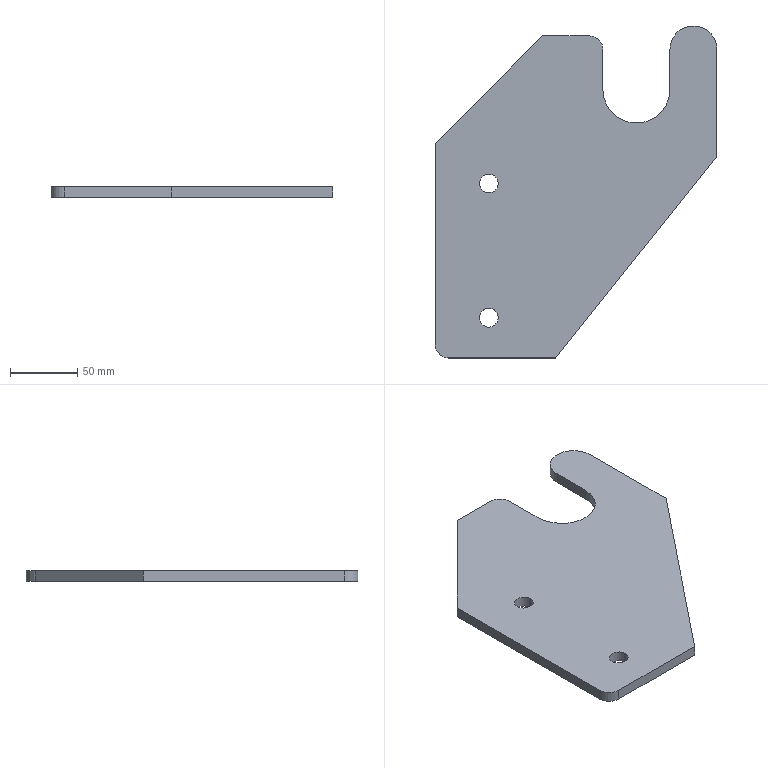Part | SolidWorks | features Extrusion 1 | 1 solid | 18 faces | box 210 x 247.5 x 8 mm | volume 279988 mm3 | plane 10 | cylinder 8 | commonest cylinder face diameters 14 x4 20 x2 35 x1 50 x1
STEP:
#1=CARTESIAN_POINT('',(33.,30.,8.));
#2=VERTEX_POINT('',#1);
#3=CARTESIAN_POINT('',(47.,30.,8.));
#4=VERTEX_POINT('',#3);
#5=CARTESIAN_POINT('',(40.,30.,8.));
#6=DIRECTION('',(0.,0.,1.));
#7=DIRECTION('',(1.,0.,0.));
#8=AXIS2_PLACEMENT_3D('',#5,#6,#7);
#9=CIRCLE('',#8,7.);
#10=EDGE_CURVE('',#2,#4,#9,.T.);
#11=ORIENTED_EDGE('',*,*,#10,.T.);
#12=CARTESIAN_POINT('',(47.,30.,0.));
#13=VERTEX_POINT('',#12);
#14=CARTESIAN_POINT('',(47.,30.,8.));
#15=DIRECTION('',(0.,0.,-1.));
#16=VECTOR('',#15,1000.);
#17=LINE('',#14,#16);
#18=EDGE_CURVE('',#4,#13,#17,.T.);
#19=ORIENTED_EDGE('',*,*,#18,.T.);
#20=CARTESIAN_POINT('',(33.,30.,0.));
#21=VERTEX_POINT('',#20);
#22=CARTESIAN_POINT('',(40.,30.,0.));
#23=DIRECTION('',(0.,0.,1.));
#24=DIRECTION('',(1.,0.,0.));
#25=AXIS2_PLACEMENT_3D('',#22,#23,#24);
#26=CIRCLE('',#25,7.);
#27=EDGE_CURVE('',#21,#13,#26,.T.);
#28=ORIENTED_EDGE('',*,*,#27,.F.);
#29=CARTESIAN_POINT('',(33.,30.,8.));
#30=DIRECTION('',(0.,0.,-1.));
#31=VECTOR('',#30,1000.);
#32=LINE('',#29,#31);
#33=EDGE_CURVE('',#2,#21,#32,.T.);
#34=ORIENTED_EDGE('',*,*,#33,.F.);
#35=EDGE_LOOP('',(#11,#19,#28,#34));
#36=FACE_OUTER_BOUND('',#35,.T.);
#37=CARTESIAN_POINT('',(40.,30.,8.));
#38=DIRECTION('',(0.,0.,-1.));
#39=DIRECTION('',(-1.,0.,0.));
#40=AXIS2_PLACEMENT_3D('',#37,#38,#39);
#41=CYLINDRICAL_SURFACE('',#40,7.);
#42=ADVANCED_FACE('',(#36),#41,.F.);
#43=CARTESIAN_POINT('',(33.,130.,8.));
#44=VERTEX_POINT('',#43);
#45=CARTESIAN_POINT('',(47.,130.,8.));
#46=VERTEX_POINT('',#45);
#47=CARTESIAN_POINT('',(40.,130.,8.));
#48=DIRECTION('',(0.,0.,1.));
#49=DIRECTION('',(1.,0.,0.));
#50=AXIS2_PLACEMENT_3D('',#47,#48,#49);
#51=CIRCLE('',#50,7.);
#52=EDGE_CURVE('',#44,#46,#51,.T.);
#53=ORIENTED_EDGE('',*,*,#52,.T.);
#54=CARTESIAN_POINT('',(47.,130.,0.));
#55=VERTEX_POINT('',#54);
#56=CARTESIAN_POINT('',(47.,130.,8.));
#57=DIRECTION('',(0.,0.,-1.));
#58=VECTOR('',#57,1000.);
#59=LINE('',#56,#58);
#60=EDGE_CURVE('',#46,#55,#59,.T.);
#61=ORIENTED_EDGE('',*,*,#60,.T.);
#62=CARTESIAN_POINT('',(33.,130.,0.));
#63=VERTEX_POINT('',#62);
#64=CARTESIAN_POINT('',(40.,130.,0.));
#65=DIRECTION('',(0.,0.,1.));
#66=DIRECTION('',(1.,0.,0.));
#67=AXIS2_PLACEMENT_3D('',#64,#65,#66);
#68=CIRCLE('',#67,7.);
#69=EDGE_CURVE('',#63,#55,#68,.T.);
#70=ORIENTED_EDGE('',*,*,#69,.F.);
#71=CARTESIAN_POINT('',(33.,130.,8.));
#72=DIRECTION('',(0.,0.,-1.));
#73=VECTOR('',#72,1000.);
#74=LINE('',#71,#73);
#75=EDGE_CURVE('',#44,#63,#74,.T.);
#76=ORIENTED_EDGE('',*,*,#75,.F.);
#77=EDGE_LOOP('',(#53,#61,#70,#76));
#78=FACE_OUTER_BOUND('',#77,.T.);
#79=CARTESIAN_POINT('',(40.,130.,8.));
#80=DIRECTION('',(0.,0.,-1.));
#81=DIRECTION('',(-1.,0.,0.));
#82=AXIS2_PLACEMENT_3D('',#79,#80,#81);
#83=CYLINDRICAL_SURFACE('',#82,7.);
#84=ADVANCED_FACE('',(#78),#83,.F.);
#85=ORIENTED_EDGE('',*,*,#52,.F.);
#86=CARTESIAN_POINT('',(40.,130.,8.));
#87=DIRECTION('',(0.,0.,1.));
#88=DIRECTION('',(1.,0.,0.));
#89=AXIS2_PLACEMENT_3D('',#86,#87,#88);
#90=CIRCLE('',#89,7.);
#91=EDGE_CURVE('',#46,#44,#90,.T.);
#92=ORIENTED_EDGE('',*,*,#91,.F.);
#93=EDGE_LOOP('',(#85,#92));
#94=FACE_BOUND('',#93,.T.);
#95=CARTESIAN_POINT('',(90.,0.,8.));
#96=VERTEX_POINT('',#95);
#97=CARTESIAN_POINT('',(210.,150.,8.));
#98=VERTEX_POINT('',#97);
#99=CARTESIAN_POINT('',(90.,0.,8.));
#100=DIRECTION('',(0.6247,0.7809,0.));
#101=VECTOR('',#100,1000.);
#102=LINE('',#99,#101);
#103=EDGE_CURVE('',#96,#98,#102,.T.);
#104=ORIENTED_EDGE('',*,*,#103,.T.);
#105=CARTESIAN_POINT('',(210.,230.,8.));
#106=VERTEX_POINT('',#105);
#107=CARTESIAN_POINT('',(210.,230.,8.));
#108=DIRECTION('',(0.,1.,0.));
#109=VECTOR('',#108,1000.);
#110=LINE('',#107,#109);
#111=EDGE_CURVE('',#98,#106,#110,.T.);
#112=ORIENTED_EDGE('',*,*,#111,.T.);
#113=CARTESIAN_POINT('',(175.,230.,8.));
#114=VERTEX_POINT('',#113);
#115=CARTESIAN_POINT('',(192.5,230.,8.));
#116=DIRECTION('',(0.,0.,1.));
#117=DIRECTION('',(1.,0.,0.));
#118=AXIS2_PLACEMENT_3D('',#115,#116,#117);
#119=CIRCLE('',#118,17.5);
#120=EDGE_CURVE('',#106,#114,#119,.T.);
#121=ORIENTED_EDGE('',*,*,#120,.T.);
#122=CARTESIAN_POINT('',(175.,200.,8.));
#123=VERTEX_POINT('',#122);
#124=CARTESIAN_POINT('',(175.,230.,8.));
#125=DIRECTION('',(0.,-1.,0.));
#126=VECTOR('',#125,1000.);
#127=LINE('',#124,#126);
#128=EDGE_CURVE('',#114,#123,#127,.T.);
#129=ORIENTED_EDGE('',*,*,#128,.T.);
#130=CARTESIAN_POINT('',(125.,200.,8.));
#131=VERTEX_POINT('',#130);
#132=CARTESIAN_POINT('',(150.,200.,8.));
#133=DIRECTION('',(0.,0.,-1.));
#134=DIRECTION('',(1.,0.,0.));
#135=AXIS2_PLACEMENT_3D('',#132,#133,#134);
#136=CIRCLE('',#135,25.);
#137=EDGE_CURVE('',#123,#131,#136,.T.);
#138=ORIENTED_EDGE('',*,*,#137,.T.);
#139=CARTESIAN_POINT('',(125.,230.,8.));
#140=VERTEX_POINT('',#139);
#141=CARTESIAN_POINT('',(125.,200.,8.));
#142=DIRECTION('',(0.,1.,0.));
#143=VECTOR('',#142,1000.);
#144=LINE('',#141,#143);
#145=EDGE_CURVE('',#131,#140,#144,.T.);
#146=ORIENTED_EDGE('',*,*,#145,.T.);
#147=CARTESIAN_POINT('',(115.,240.,8.));
#148=VERTEX_POINT('',#147);
#149=CARTESIAN_POINT('',(115.,230.,8.));
#150=DIRECTION('',(0.,0.,1.));
#151=DIRECTION('',(1.,0.,0.));
#152=AXIS2_PLACEMENT_3D('',#149,#150,#151);
#153=CIRCLE('',#152,10.);
#154=EDGE_CURVE('',#140,#148,#153,.T.);
#155=ORIENTED_EDGE('',*,*,#154,.T.);
#156=CARTESIAN_POINT('',(80.,240.,8.));
#157=VERTEX_POINT('',#156);
#158=CARTESIAN_POINT('',(115.,240.,8.));
#159=DIRECTION('',(-1.,0.,0.));
#160=VECTOR('',#159,1000.);
#161=LINE('',#158,#160);
#162=EDGE_CURVE('',#148,#157,#161,.T.);
#163=ORIENTED_EDGE('',*,*,#162,.T.);
#164=CARTESIAN_POINT('',(0.,160.,8.));
#165=VERTEX_POINT('',#164);
#166=CARTESIAN_POINT('',(80.,240.,8.));
#167=DIRECTION('',(-0.7071,-0.7071,0.));
#168=VECTOR('',#167,1000.);
#169=LINE('',#166,#168);
#170=EDGE_CURVE('',#157,#165,#169,.T.);
#171=ORIENTED_EDGE('',*,*,#170,.T.);
#172=CARTESIAN_POINT('',(0.,10.,8.));
#173=VERTEX_POINT('',#172);
#174=CARTESIAN_POINT('',(0.,160.,8.));
#175=DIRECTION('',(0.,-1.,0.));
#176=VECTOR('',#175,1000.);
#177=LINE('',#174,#176);
#178=EDGE_CURVE('',#165,#173,#177,.T.);
#179=ORIENTED_EDGE('',*,*,#178,.T.);
#180=CARTESIAN_POINT('',(10.,0.,8.));
#181=VERTEX_POINT('',#180);
#182=CARTESIAN_POINT('',(10.,10.,8.));
#183=DIRECTION('',(0.,0.,1.));
#184=DIRECTION('',(-1.,0.,0.));
#185=AXIS2_PLACEMENT_3D('',#182,#183,#184);
#186=CIRCLE('',#185,10.);
#187=EDGE_CURVE('',#173,#181,#186,.T.);
#188=ORIENTED_EDGE('',*,*,#187,.T.);
#189=CARTESIAN_POINT('',(10.,0.,8.));
#190=DIRECTION('',(1.,0.,0.));
#191=VECTOR('',#190,1000.);
#192=LINE('',#189,#191);
#193=EDGE_CURVE('',#181,#96,#192,.T.);
#194=ORIENTED_EDGE('',*,*,#193,.T.);
#195=EDGE_LOOP('',(#104,#112,#121,#129,#138,#146,#155,#163,#171,#179,#188,#194));
#196=FACE_OUTER_BOUND('',#195,.T.);
#197=ORIENTED_EDGE('',*,*,#10,.F.);
#198=CARTESIAN_POINT('',(40.,30.,8.));
#199=DIRECTION('',(0.,0.,1.));
#200=DIRECTION('',(1.,0.,0.));
#201=AXIS2_PLACEMENT_3D('',#198,#199,#200);
#202=CIRCLE('',#201,7.);
#203=EDGE_CURVE('',#4,#2,#202,.T.);
#204=ORIENTED_EDGE('',*,*,#203,.F.);
#205=EDGE_LOOP('',(#197,#204));
#206=FACE_BOUND('',#205,.T.);
#207=CARTESIAN_POINT('',(192.5,230.,8.));
#208=DIRECTION('',(0.,0.,1.));
#209=DIRECTION('',(1.,0.,0.));
#210=AXIS2_PLACEMENT_3D('',#207,#208,#209);
#211=PLANE('',#210);
#212=ADVANCED_FACE('',(#94,#196,#206),#211,.T.);
#213=CARTESIAN_POINT('',(90.,0.,0.));
#214=VERTEX_POINT('',#213);
#215=CARTESIAN_POINT('',(210.,150.,0.));
#216=VERTEX_POINT('',#215);
#217=CARTESIAN_POINT('',(90.,0.,0.));
#218=DIRECTION('',(0.6247,0.7809,0.));
#219=VECTOR('',#218,1000.);
#220=LINE('',#217,#219);
#221=EDGE_CURVE('',#214,#216,#220,.T.);
#222=ORIENTED_EDGE('',*,*,#221,.F.);
#223=CARTESIAN_POINT('',(10.,0.,0.));
#224=VERTEX_POINT('',#223);
#225=CARTESIAN_POINT('',(10.,0.,0.));
#226=DIRECTION('',(1.,0.,0.));
#227=VECTOR('',#226,1000.);
#228=LINE('',#225,#227);
#229=EDGE_CURVE('',#224,#214,#228,.T.);
#230=ORIENTED_EDGE('',*,*,#229,.F.);
#231=CARTESIAN_POINT('',(0.,10.,0.));
#232=VERTEX_POINT('',#231);
#233=CARTESIAN_POINT('',(10.,10.,0.));
#234=DIRECTION('',(0.,0.,1.));
#235=DIRECTION('',(-1.,0.,0.));
#236=AXIS2_PLACEMENT_3D('',#233,#234,#235);
#237=CIRCLE('',#236,10.);
#238=EDGE_CURVE('',#232,#224,#237,.T.);
#239=ORIENTED_EDGE('',*,*,#238,.F.);
#240=CARTESIAN_POINT('',(0.,160.,0.));
#241=VERTEX_POINT('',#240);
#242=CARTESIAN_POINT('',(0.,160.,0.));
#243=DIRECTION('',(0.,-1.,0.));
#244=VECTOR('',#243,1000.);
#245=LINE('',#242,#244);
#246=EDGE_CURVE('',#241,#232,#245,.T.);
#247=ORIENTED_EDGE('',*,*,#246,.F.);
#248=CARTESIAN_POINT('',(80.,240.,0.));
#249=VERTEX_POINT('',#248);
#250=CARTESIAN_POINT('',(80.,240.,0.));
#251=DIRECTION('',(-0.7071,-0.7071,0.));
#252=VECTOR('',#251,1000.);
#253=LINE('',#250,#252);
#254=EDGE_CURVE('',#249,#241,#253,.T.);
#255=ORIENTED_EDGE('',*,*,#254,.F.);
#256=CARTESIAN_POINT('',(115.,240.,0.));
#257=VERTEX_POINT('',#256);
#258=CARTESIAN_POINT('',(115.,240.,0.));
#259=DIRECTION('',(-1.,0.,0.));
#260=VECTOR('',#259,1000.);
#261=LINE('',#258,#260);
#262=EDGE_CURVE('',#257,#249,#261,.T.);
#263=ORIENTED_EDGE('',*,*,#262,.F.);
#264=CARTESIAN_POINT('',(125.,230.,0.));
#265=VERTEX_POINT('',#264);
#266=CARTESIAN_POINT('',(115.,230.,0.));
#267=DIRECTION('',(0.,0.,1.));
#268=DIRECTION('',(1.,0.,0.));
#269=AXIS2_PLACEMENT_3D('',#266,#267,#268);
#270=CIRCLE('',#269,10.);
#271=EDGE_CURVE('',#265,#257,#270,.T.);
#272=ORIENTED_EDGE('',*,*,#271,.F.);
#273=CARTESIAN_POINT('',(125.,200.,0.));
#274=VERTEX_POINT('',#273);
#275=CARTESIAN_POINT('',(125.,200.,0.));
#276=DIRECTION('',(0.,1.,0.));
#277=VECTOR('',#276,1000.);
#278=LINE('',#275,#277);
#279=EDGE_CURVE('',#274,#265,#278,.T.);
#280=ORIENTED_EDGE('',*,*,#279,.F.);
#281=CARTESIAN_POINT('',(175.,200.,0.));
#282=VERTEX_POINT('',#281);
#283=CARTESIAN_POINT('',(150.,200.,0.));
#284=DIRECTION('',(0.,0.,-1.));
#285=DIRECTION('',(1.,0.,0.));
#286=AXIS2_PLACEMENT_3D('',#283,#284,#285);
#287=CIRCLE('',#286,25.);
#288=EDGE_CURVE('',#282,#274,#287,.T.);
#289=ORIENTED_EDGE('',*,*,#288,.F.);
#290=CARTESIAN_POINT('',(175.,230.,0.));
#291=VERTEX_POINT('',#290);
#292=CARTESIAN_POINT('',(175.,230.,0.));
#293=DIRECTION('',(0.,-1.,0.));
#294=VECTOR('',#293,1000.);
#295=LINE('',#292,#294);
#296=EDGE_CURVE('',#291,#282,#295,.T.);
#297=ORIENTED_EDGE('',*,*,#296,.F.);
#298=CARTESIAN_POINT('',(210.,230.,0.));
#299=VERTEX_POINT('',#298);
#300=CARTESIAN_POINT('',(192.5,230.,0.));
#301=DIRECTION('',(0.,0.,1.));
#302=DIRECTION('',(1.,0.,0.));
#303=AXIS2_PLACEMENT_3D('',#300,#301,#302);
#304=CIRCLE('',#303,17.5);
#305=EDGE_CURVE('',#299,#291,#304,.T.);
#306=ORIENTED_EDGE('',*,*,#305,.F.);
#307=CARTESIAN_POINT('',(210.,230.,0.));
#308=DIRECTION('',(0.,1.,0.));
#309=VECTOR('',#308,1000.);
#310=LINE('',#307,#309);
#311=EDGE_CURVE('',#216,#299,#310,.T.);
#312=ORIENTED_EDGE('',*,*,#311,.F.);
#313=EDGE_LOOP('',(#222,#230,#239,#247,#255,#263,#272,#280,#289,#297,#306,#312));
#314=FACE_OUTER_BOUND('',#313,.T.);
#315=ORIENTED_EDGE('',*,*,#69,.T.);
#316=CARTESIAN_POINT('',(40.,130.,0.));
#317=DIRECTION('',(0.,0.,1.));
#318=DIRECTION('',(1.,0.,0.));
#319=AXIS2_PLACEMENT_3D('',#316,#317,#318);
#320=CIRCLE('',#319,7.);
#321=EDGE_CURVE('',#55,#63,#320,.T.);
#322=ORIENTED_EDGE('',*,*,#321,.T.);
#323=EDGE_LOOP('',(#315,#322));
#324=FACE_BOUND('',#323,.T.);
#325=ORIENTED_EDGE('',*,*,#27,.T.);
#326=CARTESIAN_POINT('',(40.,30.,0.));
#327=DIRECTION('',(0.,0.,1.));
#328=DIRECTION('',(1.,0.,0.));
#329=AXIS2_PLACEMENT_3D('',#326,#327,#328);
#330=CIRCLE('',#329,7.);
#331=EDGE_CURVE('',#13,#21,#330,.T.);
#332=ORIENTED_EDGE('',*,*,#331,.T.);
#333=EDGE_LOOP('',(#325,#332));
#334=FACE_BOUND('',#333,.T.);
#335=CARTESIAN_POINT('',(192.5,230.,0.));
#336=DIRECTION('',(0.,0.,1.));
#337=DIRECTION('',(1.,0.,0.));
#338=AXIS2_PLACEMENT_3D('',#335,#336,#337);
#339=PLANE('',#338);
#340=ADVANCED_FACE('',(#314,#324,#334),#339,.F.);
#341=ORIENTED_EDGE('',*,*,#221,.T.);
#342=CARTESIAN_POINT('',(210.,150.,8.));
#343=DIRECTION('',(0.,0.,-1.));
#344=VECTOR('',#343,1000.);
#345=LINE('',#342,#344);
#346=EDGE_CURVE('',#98,#216,#345,.T.);
#347=ORIENTED_EDGE('',*,*,#346,.F.);
#348=ORIENTED_EDGE('',*,*,#103,.F.);
#349=CARTESIAN_POINT('',(90.,0.,8.));
#350=DIRECTION('',(0.,0.,-1.));
#351=VECTOR('',#350,1000.);
#352=LINE('',#349,#351);
#353=EDGE_CURVE('',#96,#214,#352,.T.);
#354=ORIENTED_EDGE('',*,*,#353,.T.);
#355=EDGE_LOOP('',(#341,#347,#348,#354));
#356=FACE_OUTER_BOUND('',#355,.T.);
#357=CARTESIAN_POINT('',(90.,0.,8.));
#358=DIRECTION('',(-0.7809,0.6247,0.));
#359=DIRECTION('',(-0.6247,-0.7809,0.));
#360=AXIS2_PLACEMENT_3D('',#357,#358,#359);
#361=PLANE('',#360);
#362=ADVANCED_FACE('',(#356),#361,.F.);
#363=ORIENTED_EDGE('',*,*,#311,.T.);
#364=CARTESIAN_POINT('',(210.,230.,8.));
#365=DIRECTION('',(0.,0.,-1.));
#366=VECTOR('',#365,1000.);
#367=LINE('',#364,#366);
#368=EDGE_CURVE('',#106,#299,#367,.T.);
#369=ORIENTED_EDGE('',*,*,#368,.F.);
#370=ORIENTED_EDGE('',*,*,#111,.F.);
#371=ORIENTED_EDGE('',*,*,#346,.T.);
#372=EDGE_LOOP('',(#363,#369,#370,#371));
#373=FACE_OUTER_BOUND('',#372,.T.);
#374=CARTESIAN_POINT('',(210.,230.,8.));
#375=DIRECTION('',(-1.,0.,0.));
#376=DIRECTION('',(0.,-1.,0.));
#377=AXIS2_PLACEMENT_3D('',#374,#375,#376);
#378=PLANE('',#377);
#379=ADVANCED_FACE('',(#373),#378,.F.);
#380=ORIENTED_EDGE('',*,*,#305,.T.);
#381=CARTESIAN_POINT('',(175.,230.,8.));
#382=DIRECTION('',(0.,0.,-1.));
#383=VECTOR('',#382,1000.);
#384=LINE('',#381,#383);
#385=EDGE_CURVE('',#114,#291,#384,.T.);
#386=ORIENTED_EDGE('',*,*,#385,.F.);
#387=ORIENTED_EDGE('',*,*,#120,.F.);
#388=ORIENTED_EDGE('',*,*,#368,.T.);
#389=EDGE_LOOP('',(#380,#386,#387,#388));
#390=FACE_OUTER_BOUND('',#389,.T.);
#391=CARTESIAN_POINT('',(192.5,230.,8.));
#392=DIRECTION('',(0.,0.,-1.));
#393=DIRECTION('',(-1.,0.,0.));
#394=AXIS2_PLACEMENT_3D('',#391,#392,#393);
#395=CYLINDRICAL_SURFACE('',#394,17.5);
#396=ADVANCED_FACE('',(#390),#395,.T.);
#397=ORIENTED_EDGE('',*,*,#296,.T.);
#398=CARTESIAN_POINT('',(175.,200.,8.));
#399=DIRECTION('',(0.,0.,-1.));
#400=VECTOR('',#399,1000.);
#401=LINE('',#398,#400);
#402=EDGE_CURVE('',#123,#282,#401,.T.);
#403=ORIENTED_EDGE('',*,*,#402,.F.);
#404=ORIENTED_EDGE('',*,*,#128,.F.);
#405=ORIENTED_EDGE('',*,*,#385,.T.);
#406=EDGE_LOOP('',(#397,#403,#404,#405));
#407=FACE_OUTER_BOUND('',#406,.T.);
#408=CARTESIAN_POINT('',(175.,230.,8.));
#409=DIRECTION('',(1.,0.,0.));
#410=DIRECTION('',(0.,1.,0.));
#411=AXIS2_PLACEMENT_3D('',#408,#409,#410);
#412=PLANE('',#411);
#413=ADVANCED_FACE('',(#407),#412,.F.);
#414=ORIENTED_EDGE('',*,*,#288,.T.);
#415=CARTESIAN_POINT('',(125.,200.,8.));
#416=DIRECTION('',(0.,0.,-1.));
#417=VECTOR('',#416,1000.);
#418=LINE('',#415,#417);
#419=EDGE_CURVE('',#131,#274,#418,.T.);
#420=ORIENTED_EDGE('',*,*,#419,.F.);
#421=ORIENTED_EDGE('',*,*,#137,.F.);
#422=ORIENTED_EDGE('',*,*,#402,.T.);
#423=EDGE_LOOP('',(#414,#420,#421,#422));
#424=FACE_OUTER_BOUND('',#423,.T.);
#425=CARTESIAN_POINT('',(150.,200.,8.));
#426=DIRECTION('',(0.,0.,-1.));
#427=DIRECTION('',(-1.,0.,0.));
#428=AXIS2_PLACEMENT_3D('',#425,#426,#427);
#429=CYLINDRICAL_SURFACE('',#428,25.);
#430=ADVANCED_FACE('',(#424),#429,.F.);
#431=ORIENTED_EDGE('',*,*,#279,.T.);
#432=CARTESIAN_POINT('',(125.,230.,8.));
#433=DIRECTION('',(0.,0.,-1.));
#434=VECTOR('',#433,1000.);
#435=LINE('',#432,#434);
#436=EDGE_CURVE('',#140,#265,#435,.T.);
#437=ORIENTED_EDGE('',*,*,#436,.F.);
#438=ORIENTED_EDGE('',*,*,#145,.F.);
#439=ORIENTED_EDGE('',*,*,#419,.T.);
#440=EDGE_LOOP('',(#431,#437,#438,#439));
#441=FACE_OUTER_BOUND('',#440,.T.);
#442=CARTESIAN_POINT('',(125.,200.,8.));
#443=DIRECTION('',(-1.,0.,0.));
#444=DIRECTION('',(0.,-1.,0.));
#445=AXIS2_PLACEMENT_3D('',#442,#443,#444);
#446=PLANE('',#445);
#447=ADVANCED_FACE('',(#441),#446,.F.);
#448=ORIENTED_EDGE('',*,*,#271,.T.);
#449=CARTESIAN_POINT('',(115.,240.,8.));
#450=DIRECTION('',(0.,0.,-1.));
#451=VECTOR('',#450,1000.);
#452=LINE('',#449,#451);
#453=EDGE_CURVE('',#148,#257,#452,.T.);
#454=ORIENTED_EDGE('',*,*,#453,.F.);
#455=ORIENTED_EDGE('',*,*,#154,.F.);
#456=ORIENTED_EDGE('',*,*,#436,.T.);
#457=EDGE_LOOP('',(#448,#454,#455,#456));
#458=FACE_OUTER_BOUND('',#457,.T.);
#459=CARTESIAN_POINT('',(115.,230.,8.));
#460=DIRECTION('',(0.,0.,-1.));
#461=DIRECTION('',(-1.,0.,0.));
#462=AXIS2_PLACEMENT_3D('',#459,#460,#461);
#463=CYLINDRICAL_SURFACE('',#462,10.);
#464=ADVANCED_FACE('',(#458),#463,.T.);
#465=ORIENTED_EDGE('',*,*,#262,.T.);
#466=CARTESIAN_POINT('',(80.,240.,8.));
#467=DIRECTION('',(0.,0.,-1.));
#468=VECTOR('',#467,1000.);
#469=LINE('',#466,#468);
#470=EDGE_CURVE('',#157,#249,#469,.T.);
#471=ORIENTED_EDGE('',*,*,#470,.F.);
#472=ORIENTED_EDGE('',*,*,#162,.F.);
#473=ORIENTED_EDGE('',*,*,#453,.T.);
#474=EDGE_LOOP('',(#465,#471,#472,#473));
#475=FACE_OUTER_BOUND('',#474,.T.);
#476=CARTESIAN_POINT('',(115.,240.,8.));
#477=DIRECTION('',(0.,-1.,0.));
#478=DIRECTION('',(0.,0.,-1.));
#479=AXIS2_PLACEMENT_3D('',#476,#477,#478);
#480=PLANE('',#479);
#481=ADVANCED_FACE('',(#475),#480,.F.);
#482=ORIENTED_EDGE('',*,*,#254,.T.);
#483=CARTESIAN_POINT('',(0.,160.,8.));
#484=DIRECTION('',(0.,0.,-1.));
#485=VECTOR('',#484,1000.);
#486=LINE('',#483,#485);
#487=EDGE_CURVE('',#165,#241,#486,.T.);
#488=ORIENTED_EDGE('',*,*,#487,.F.);
#489=ORIENTED_EDGE('',*,*,#170,.F.);
#490=ORIENTED_EDGE('',*,*,#470,.T.);
#491=EDGE_LOOP('',(#482,#488,#489,#490));
#492=FACE_OUTER_BOUND('',#491,.T.);
#493=CARTESIAN_POINT('',(80.,240.,8.));
#494=DIRECTION('',(0.7071,-0.7071,0.));
#495=DIRECTION('',(0.7071,0.7071,0.));
#496=AXIS2_PLACEMENT_3D('',#493,#494,#495);
#497=PLANE('',#496);
#498=ADVANCED_FACE('',(#492),#497,.F.);
#499=ORIENTED_EDGE('',*,*,#246,.T.);
#500=CARTESIAN_POINT('',(0.,10.,8.));
#501=DIRECTION('',(0.,0.,-1.));
#502=VECTOR('',#501,1000.);
#503=LINE('',#500,#502);
#504=EDGE_CURVE('',#173,#232,#503,.T.);
#505=ORIENTED_EDGE('',*,*,#504,.F.);
#506=ORIENTED_EDGE('',*,*,#178,.F.);
#507=ORIENTED_EDGE('',*,*,#487,.T.);
#508=EDGE_LOOP('',(#499,#505,#506,#507));
#509=FACE_OUTER_BOUND('',#508,.T.);
#510=CARTESIAN_POINT('',(0.,160.,8.));
#511=DIRECTION('',(1.,0.,0.));
#512=DIRECTION('',(0.,1.,0.));
#513=AXIS2_PLACEMENT_3D('',#510,#511,#512);
#514=PLANE('',#513);
#515=ADVANCED_FACE('',(#509),#514,.F.);
#516=ORIENTED_EDGE('',*,*,#238,.T.);
#517=CARTESIAN_POINT('',(10.,0.,8.));
#518=DIRECTION('',(0.,0.,-1.));
#519=VECTOR('',#518,1000.);
#520=LINE('',#517,#519);
#521=EDGE_CURVE('',#181,#224,#520,.T.);
#522=ORIENTED_EDGE('',*,*,#521,.F.);
#523=ORIENTED_EDGE('',*,*,#187,.F.);
#524=ORIENTED_EDGE('',*,*,#504,.T.);
#525=EDGE_LOOP('',(#516,#522,#523,#524));
#526=FACE_OUTER_BOUND('',#525,.T.);
#527=CARTESIAN_POINT('',(10.,10.,8.));
#528=DIRECTION('',(0.,0.,-1.));
#529=DIRECTION('',(-1.,0.,0.));
#530=AXIS2_PLACEMENT_3D('',#527,#528,#529);
#531=CYLINDRICAL_SURFACE('',#530,10.);
#532=ADVANCED_FACE('',(#526),#531,.T.);
#533=ORIENTED_EDGE('',*,*,#229,.T.);
#534=ORIENTED_EDGE('',*,*,#353,.F.);
#535=ORIENTED_EDGE('',*,*,#193,.F.);
#536=ORIENTED_EDGE('',*,*,#521,.T.);
#537=EDGE_LOOP('',(#533,#534,#535,#536));
#538=FACE_OUTER_BOUND('',#537,.T.);
#539=CARTESIAN_POINT('',(10.,0.,8.));
#540=DIRECTION('',(0.,1.,0.));
#541=DIRECTION('',(0.,0.,1.));
#542=AXIS2_PLACEMENT_3D('',#539,#540,#541);
#543=PLANE('',#542);
#544=ADVANCED_FACE('',(#538),#543,.F.);
#545=ORIENTED_EDGE('',*,*,#60,.F.);
#546=ORIENTED_EDGE('',*,*,#91,.T.);
#547=ORIENTED_EDGE('',*,*,#75,.T.);
#548=ORIENTED_EDGE('',*,*,#321,.F.);
#549=EDGE_LOOP('',(#545,#546,#547,#548));
#550=FACE_OUTER_BOUND('',#549,.T.);
#551=CARTESIAN_POINT('',(40.,130.,8.));
#552=DIRECTION('',(0.,0.,-1.));
#553=DIRECTION('',(-1.,0.,0.));
#554=AXIS2_PLACEMENT_3D('',#551,#552,#553);
#555=CYLINDRICAL_SURFACE('',#554,7.);
#556=ADVANCED_FACE('',(#550),#555,.F.);
#557=ORIENTED_EDGE('',*,*,#18,.F.);
#558=ORIENTED_EDGE('',*,*,#203,.T.);
#559=ORIENTED_EDGE('',*,*,#33,.T.);
#560=ORIENTED_EDGE('',*,*,#331,.F.);
#561=EDGE_LOOP('',(#557,#558,#559,#560));
#562=FACE_OUTER_BOUND('',#561,.T.);
#563=CARTESIAN_POINT('',(40.,30.,8.));
#564=DIRECTION('',(0.,0.,-1.));
#565=DIRECTION('',(-1.,0.,0.));
#566=AXIS2_PLACEMENT_3D('',#563,#564,#565);
#567=CYLINDRICAL_SURFACE('',#566,7.);
#568=ADVANCED_FACE('',(#562),#567,.F.);
#569=CLOSED_SHELL('',(#42,#84,#212,#340,#362,#379,#396,#413,#430,#447,#464,#481,#498,#515,#532,#544,#556,#568));
#570=MANIFOLD_SOLID_BREP('',#569);
#571=CARTESIAN_POINT('',(0.,0.,0.));
#572=DIRECTION('',(0.,0.,1.));
#573=DIRECTION('',(1.,0.,0.));
#574=AXIS2_PLACEMENT_3D('',#571,#572,#573);
#575=(LENGTH_UNIT()NAMED_UNIT(*)SI_UNIT(.MILLI.,.METRE.));
#576=UNCERTAINTY_MEASURE_WITH_UNIT(LENGTH_MEASURE(0.00001),#575,'','');
#577=(NAMED_UNIT(*)PLANE_ANGLE_UNIT()SI_UNIT($,.RADIAN.));
#578=(NAMED_UNIT(*)SI_UNIT($,.STERADIAN.)SOLID_ANGLE_UNIT());
#579=(GEOMETRIC_REPRESENTATION_CONTEXT(3)GLOBAL_UNCERTAINTY_ASSIGNED_CONTEXT((#576))GLOBAL_UNIT_ASSIGNED_CONTEXT((#575,#577,#578))REPRESENTATION_CONTEXT('',''));
#580=ADVANCED_BREP_SHAPE_REPRESENTATION('',(#570,#574),#579);